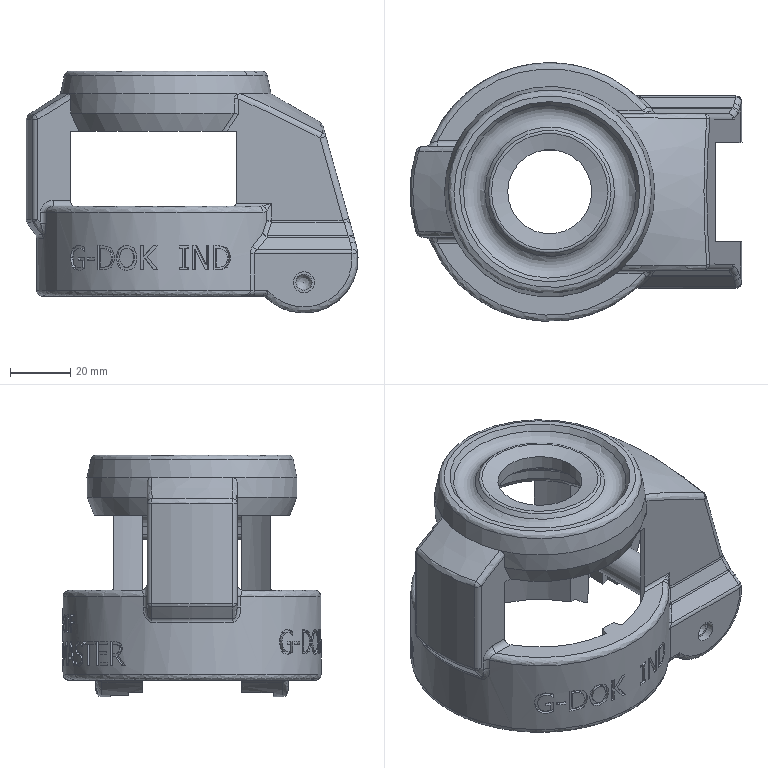Part | STEP file | 1 solid | 586 faces | box 110.5 x 86 x 80.5 mm | volume 156144 mm3 | spline 251 | plane 204 | cylinder 108 | cone 12 | torus 5 | sphere 4 | other 2 | commonest cylinder face diameters 4 x34 84 x24 86 x12 1 x8 2 x6 7 x4